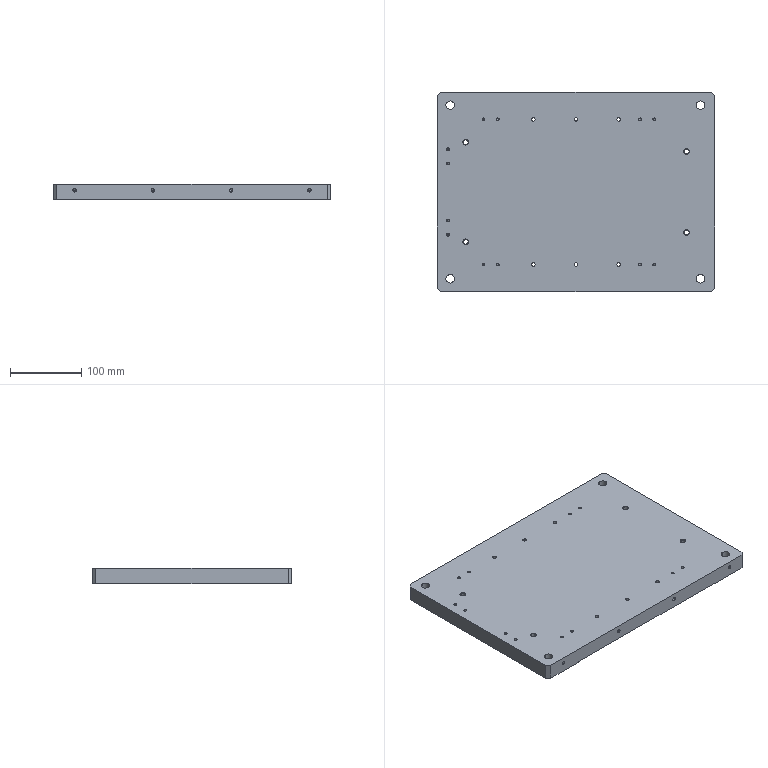NC program | NX | posted with a generic post | part box 390 x 280 x 22 mm
Lines 1 to 1875 of 1943, first 1630 of 1861 lines:
N10 G17 G21 G94 G90
(FLOOR_WALL , TOOL : D20R0.8)
N12 T01 M6
N14 G54
N16 G17 G0 G90 X-210.5 Y142.499 S7500 M3
N18 G43 Z30. H1
N20 Z3.
N22 G94 G1 Z0. F1350.
N24 X-207.5
N26 X207.5
N28 Y132.583
N30 X-207.5
N32 Y122.668
N34 X207.5
N36 Y112.752
N38 X-207.5
N40 Y102.836
N42 X207.5
N44 Y92.921
N46 X-207.5
N48 Y83.005
N50 X207.5
N52 Y73.089
N54 X-207.5
N56 Y63.174
N58 X207.5
N60 Y53.258
N62 X-207.5
N64 Y43.342
N66 X207.5
N68 Y33.427
N70 X-207.5
N72 Y23.511
N74 X207.5
N76 Y13.595
N78 X-207.5
N80 Y3.68
N82 X207.5
N84 Y-6.236
N86 X-207.5
N88 Y-16.152
N90 X207.5
N92 Y-26.068
N94 X-207.5
N96 Y-35.983
N98 X207.5
N100 Y-45.899
N102 X-207.5
N104 Y-55.815
N106 X207.5
N108 Y-65.73
N110 X-207.5
N112 Y-75.646
N114 X207.5
N116 Y-85.562
N118 X-207.5
N120 Y-95.477
N122 X207.5
N124 Y-105.393
N126 X-207.5
N128 Y-115.309
N130 X207.5
N132 Y-125.224
N134 X-207.5
N136 Y-135.14
N138 X207.5
N140 X210.5
N142 Z3.
N144 G0 Z30.
N146 M5
(ZLEVEL_PROFILE_1 , TOOL : D6)
N148 T06 M6
N150 G54
N152 G17 G0 G90 X34.282 Y-143.1 S9500 M3
N154 G43 Z30. H6
N156 Z1.5
N158 G94 G1 X0. Z-0.297 F1000.
N160 X-190. F3000.
N162 G2 X-192.192 Y-142.192 R3.1
N164 G1 X-197.192 Y-137.192
N166 G2 X-198.1 Y-135. R3.1
N168 G1 Y135.
N170 G2 X-197.192 Y137.192 R3.1
N172 G1 X-192.192 Y142.192
N174 G2 X-190. Y143.1 R3.1
N176 G1 X190.
N178 G2 X192.192 Y142.192 R3.1
N180 G1 X197.192 Y137.192
N182 G2 X198.1 Y135. R3.1
N184 G1 Y-135.
N186 G2 X197.192 Y-137.192 R3.1
N188 G1 X192.192 Y-142.192
N190 G2 X190. Y-143.1 R3.1
N192 G1 X0.
N194 X-16.993 Z-0.593
N196 X-190.
N198 G2 X-192.192 Y-142.192 R3.1
N200 G1 X-197.192 Y-137.192
N202 G2 X-198.1 Y-135. R3.1
N204 G1 Y135.
N206 G2 X-197.192 Y137.192 R3.1
N208 G1 X-192.192 Y142.192
N210 G2 X-190. Y143.1 R3.1
N212 G1 X190.
N214 G2 X192.192 Y142.192 R3.1
N216 G1 X197.192 Y137.192
N218 G2 X198.1 Y135. R3.1
N220 G1 Y-135.
N222 G2 X197.192 Y-137.192 R3.1
N224 G1 X192.192 Y-142.192
N226 G2 X190. Y-143.1 R3.1
N228 G1 X0.
N230 X-16.993 Z-0.89
N232 X-190.
N234 G2 X-192.192 Y-142.192 R3.1
N236 G1 X-197.192 Y-137.192
N238 G2 X-198.1 Y-135. R3.1
N240 G1 Y135.
N242 G2 X-197.192 Y137.192 R3.1
N244 G1 X-192.192 Y142.192
N246 G2 X-190. Y143.1 R3.1
N248 G1 X190.
N250 G2 X192.192 Y142.192 R3.1
N252 G1 X197.192 Y137.192
N254 G2 X198.1 Y135. R3.1
N256 G1 Y-135.
N258 G2 X197.192 Y-137.192 R3.1
N260 G1 X192.192 Y-142.192
N262 G2 X190. Y-143.1 R3.1
N264 G1 X0.
N266 X-16.993 Z-1.186
N268 X-190.
N270 G2 X-192.192 Y-142.192 R3.1
N272 G1 X-197.192 Y-137.192
N274 G2 X-198.1 Y-135. R3.1
N276 G1 Y135.
N278 G2 X-197.192 Y137.192 R3.1
N280 G1 X-192.192 Y142.192
N282 G2 X-190. Y143.1 R3.1
N284 G1 X190.
N286 G2 X192.192 Y142.192 R3.1
N288 G1 X197.192 Y137.192
N290 G2 X198.1 Y135. R3.1
N292 G1 Y-135.
N294 G2 X197.192 Y-137.192 R3.1
N296 G1 X192.192 Y-142.192
N298 G2 X190. Y-143.1 R3.1
N300 G1 X0.
N302 X-16.993 Z-1.483
N304 X-190.
N306 G2 X-192.192 Y-142.192 R3.1
N308 G1 X-197.192 Y-137.192
N310 G2 X-198.1 Y-135. R3.1
N312 G1 Y135.
N314 G2 X-197.192 Y137.192 R3.1
N316 G1 X-192.192 Y142.192
N318 G2 X-190. Y143.1 R3.1
N320 G1 X190.
N322 G2 X192.192 Y142.192 R3.1
N324 G1 X197.192 Y137.192
N326 G2 X198.1 Y135. R3.1
N328 G1 Y-135.
N330 G2 X197.192 Y-137.192 R3.1
N332 G1 X192.192 Y-142.192
N334 G2 X190. Y-143.1 R3.1
N336 G1 X0.
N338 X-16.993 Z-1.78
N340 X-190.
N342 G2 X-192.192 Y-142.192 R3.1
N344 G1 X-197.192 Y-137.192
N346 G2 X-198.1 Y-135. R3.1
N348 G1 Y135.
N350 G2 X-197.192 Y137.192 R3.1
N352 G1 X-192.192 Y142.192
N354 G2 X-190. Y143.1 R3.1
N356 G1 X190.
N358 G2 X192.192 Y142.192 R3.1
N360 G1 X197.192 Y137.192
N362 G2 X198.1 Y135. R3.1
N364 G1 Y-135.
N366 G2 X197.192 Y-137.192 R3.1
N368 G1 X192.192 Y-142.192
N370 G2 X190. Y-143.1 R3.1
N372 G1 X0.
N374 X-16.993 Z-2.076
N376 X-190.
N378 G2 X-192.192 Y-142.192 R3.1
N380 G1 X-197.192 Y-137.192
N382 G2 X-198.1 Y-135. R3.1
N384 G1 Y135.
N386 G2 X-197.192 Y137.192 R3.1
N388 G1 X-192.192 Y142.192
N390 G2 X-190. Y143.1 R3.1
N392 G1 X190.
N394 G2 X192.192 Y142.192 R3.1
N396 G1 X197.192 Y137.192
N398 G2 X198.1 Y135. R3.1
N400 G1 Y-135.
N402 G2 X197.192 Y-137.192 R3.1
N404 G1 X192.192 Y-142.192
N406 G2 X190. Y-143.1 R3.1
N408 G1 X0.
N410 X-16.993 Z-2.373
N412 X-190.
N414 G2 X-192.192 Y-142.192 R3.1
N416 G1 X-197.192 Y-137.192
N418 G2 X-198.1 Y-135. R3.1
N420 G1 Y135.
N422 G2 X-197.192 Y137.192 R3.1
N424 G1 X-192.192 Y142.192
N426 G2 X-190. Y143.1 R3.1
N428 G1 X190.
N430 G2 X192.192 Y142.192 R3.1
N432 G1 X197.192 Y137.192
N434 G2 X198.1 Y135. R3.1
N436 G1 Y-135.
N438 G2 X197.192 Y-137.192 R3.1
N440 G1 X192.192 Y-142.192
N442 G2 X190. Y-143.1 R3.1
N444 G1 X0.
N446 X-16.993 Z-2.67
N448 X-190.
N450 G2 X-192.192 Y-142.192 R3.1
N452 G1 X-197.192 Y-137.192
N454 G2 X-198.1 Y-135. R3.1
N456 G1 Y135.
N458 G2 X-197.192 Y137.192 R3.1
N460 G1 X-192.192 Y142.192
N462 G2 X-190. Y143.1 R3.1
N464 G1 X190.
N466 G2 X192.192 Y142.192 R3.1
N468 G1 X197.192 Y137.192
N470 G2 X198.1 Y135. R3.1
N472 G1 Y-135.
N474 G2 X197.192 Y-137.192 R3.1
N476 G1 X192.192 Y-142.192
N478 G2 X190. Y-143.1 R3.1
N480 G1 X0.
N482 X-16.993 Z-2.966
N484 X-190.
N486 G2 X-192.192 Y-142.192 R3.1
N488 G1 X-197.192 Y-137.192
N490 G2 X-198.1 Y-135. R3.1
N492 G1 Y135.
N494 G2 X-197.192 Y137.192 R3.1
N496 G1 X-192.192 Y142.192
N498 G2 X-190. Y143.1 R3.1
N500 G1 X190.
N502 G2 X192.192 Y142.192 R3.1
N504 G1 X197.192 Y137.192
N506 G2 X198.1 Y135. R3.1
N508 G1 Y-135.
N510 G2 X197.192 Y-137.192 R3.1
N512 G1 X192.192 Y-142.192
N514 G2 X190. Y-143.1 R3.1
N516 G1 X0.
N518 X-16.993 Z-3.263
N520 X-190.
N522 G2 X-192.192 Y-142.192 R3.1
N524 G1 X-197.192 Y-137.192
N526 G2 X-198.1 Y-135. R3.1
N528 G1 Y135.
N530 G2 X-197.192 Y137.192 R3.1
N532 G1 X-192.192 Y142.192
N534 G2 X-190. Y143.1 R3.1
N536 G1 X190.
N538 G2 X192.192 Y142.192 R3.1
N540 G1 X197.192 Y137.192
N542 G2 X198.1 Y135. R3.1
N544 G1 Y-135.
N546 G2 X197.192 Y-137.192 R3.1
N548 G1 X192.192 Y-142.192
N550 G2 X190. Y-143.1 R3.1
N552 G1 X0.
N554 X-16.993 Z-3.559
N556 X-190.
N558 G2 X-192.192 Y-142.192 R3.1
N560 G1 X-197.192 Y-137.192
N562 G2 X-198.1 Y-135. R3.1
N564 G1 Y135.
N566 G2 X-197.192 Y137.192 R3.1
N568 G1 X-192.192 Y142.192
N570 G2 X-190. Y143.1 R3.1
N572 G1 X190.
N574 G2 X192.192 Y142.192 R3.1
N576 G1 X197.192 Y137.192
N578 G2 X198.1 Y135. R3.1
N580 G1 Y-135.
N582 G2 X197.192 Y-137.192 R3.1
N584 G1 X192.192 Y-142.192
N586 G2 X190. Y-143.1 R3.1
N588 G1 X0.
N590 X-16.993 Z-3.856
N592 X-190.
N594 G2 X-192.192 Y-142.192 R3.1
N596 G1 X-197.192 Y-137.192
N598 G2 X-198.1 Y-135. R3.1
N600 G1 Y135.
N602 G2 X-197.192 Y137.192 R3.1
N604 G1 X-192.192 Y142.192
N606 G2 X-190. Y143.1 R3.1
N608 G1 X190.
N610 G2 X192.192 Y142.192 R3.1
N612 G1 X197.192 Y137.192
N614 G2 X198.1 Y135. R3.1
N616 G1 Y-135.
N618 G2 X197.192 Y-137.192 R3.1
N620 G1 X192.192 Y-142.192
N622 G2 X190. Y-143.1 R3.1
N624 G1 X0.
N626 X-16.993 Z-4.153
N628 X-190.
N630 G2 X-192.192 Y-142.192 R3.1
N632 G1 X-197.192 Y-137.192
N634 G2 X-198.1 Y-135. R3.1
N636 G1 Y135.
N638 G2 X-197.192 Y137.192 R3.1
N640 G1 X-192.192 Y142.192
N642 G2 X-190. Y143.1 R3.1
N644 G1 X190.
N646 G2 X192.192 Y142.192 R3.1
N648 G1 X197.192 Y137.192
N650 G2 X198.1 Y135. R3.1
N652 G1 Y-135.
N654 G2 X197.192 Y-137.192 R3.1
N656 G1 X192.192 Y-142.192
N658 G2 X190. Y-143.1 R3.1
N660 G1 X0.
N662 X-16.993 Z-4.449
N664 X-190.
N666 G2 X-192.192 Y-142.192 R3.1
N668 G1 X-197.192 Y-137.192
N670 G2 X-198.1 Y-135. R3.1
N672 G1 Y135.
N674 G2 X-197.192 Y137.192 R3.1
N676 G1 X-192.192 Y142.192
N678 G2 X-190. Y143.1 R3.1
N680 G1 X190.
N682 G2 X192.192 Y142.192 R3.1
N684 G1 X197.192 Y137.192
N686 G2 X198.1 Y135. R3.1
N688 G1 Y-135.
N690 G2 X197.192 Y-137.192 R3.1
N692 G1 X192.192 Y-142.192
N694 G2 X190. Y-143.1 R3.1
N696 G1 X0.
N698 X-16.993 Z-4.746
N700 X-190.
N702 G2 X-192.192 Y-142.192 R3.1
N704 G1 X-197.192 Y-137.192
N706 G2 X-198.1 Y-135. R3.1
N708 G1 Y135.
N710 G2 X-197.192 Y137.192 R3.1
N712 G1 X-192.192 Y142.192
N714 G2 X-190. Y143.1 R3.1
N716 G1 X190.
N718 G2 X192.192 Y142.192 R3.1
N720 G1 X197.192 Y137.192
N722 G2 X198.1 Y135. R3.1
N724 G1 Y-135.
N726 G2 X197.192 Y-137.192 R3.1
N728 G1 X192.192 Y-142.192
N730 G2 X190. Y-143.1 R3.1
N732 G1 X0.
N734 X-16.993 Z-5.043
N736 X-190.
N738 G2 X-192.192 Y-142.192 R3.1
N740 G1 X-197.192 Y-137.192
N742 G2 X-198.1 Y-135. R3.1
N744 G1 Y135.
N746 G2 X-197.192 Y137.192 R3.1
N748 G1 X-192.192 Y142.192
N750 G2 X-190. Y143.1 R3.1
N752 G1 X190.
N754 G2 X192.192 Y142.192 R3.1
N756 G1 X197.192 Y137.192
N758 G2 X198.1 Y135. R3.1
N760 G1 Y-135.
N762 G2 X197.192 Y-137.192 R3.1
N764 G1 X192.192 Y-142.192
N766 G2 X190. Y-143.1 R3.1
N768 G1 X0.
N770 X-16.993 Z-5.339
N772 X-190.
N774 G2 X-192.192 Y-142.192 R3.1
N776 G1 X-197.192 Y-137.192
N778 G2 X-198.1 Y-135. R3.1
N780 G1 Y135.
N782 G2 X-197.192 Y137.192 R3.1
N784 G1 X-192.192 Y142.192
N786 G2 X-190. Y143.1 R3.1
N788 G1 X190.
N790 G2 X192.192 Y142.192 R3.1
N792 G1 X197.192 Y137.192
N794 G2 X198.1 Y135. R3.1
N796 G1 Y-135.
N798 G2 X197.192 Y-137.192 R3.1
N800 G1 X192.192 Y-142.192
N802 G2 X190. Y-143.1 R3.1
N804 G1 X0.
N806 X-16.993 Z-5.636
N808 X-190.
N810 G2 X-192.192 Y-142.192 R3.1
N812 G1 X-197.192 Y-137.192
N814 G2 X-198.1 Y-135. R3.1
N816 G1 Y135.
N818 G2 X-197.192 Y137.192 R3.1
N820 G1 X-192.192 Y142.192
N822 G2 X-190. Y143.1 R3.1
N824 G1 X190.
N826 G2 X192.192 Y142.192 R3.1
N828 G1 X197.192 Y137.192
N830 G2 X198.1 Y135. R3.1
N832 G1 Y-135.
N834 G2 X197.192 Y-137.192 R3.1
N836 G1 X192.192 Y-142.192
N838 G2 X190. Y-143.1 R3.1
N840 G1 X0.
N842 X-16.993 Z-5.932
N844 X-190.
N846 G2 X-192.192 Y-142.192 R3.1
N848 G1 X-197.192 Y-137.192
N850 G2 X-198.1 Y-135. R3.1
N852 G1 Y135.
N854 G2 X-197.192 Y137.192 R3.1
N856 G1 X-192.192 Y142.192
N858 G2 X-190. Y143.1 R3.1
N860 G1 X190.
N862 G2 X192.192 Y142.192 R3.1
N864 G1 X197.192 Y137.192
N866 G2 X198.1 Y135. R3.1
N868 G1 Y-135.
N870 G2 X197.192 Y-137.192 R3.1
N872 G1 X192.192 Y-142.192
N874 G2 X190. Y-143.1 R3.1
N876 G1 X0.
N878 X-16.993 Z-6.229
N880 X-190.
N882 G2 X-192.192 Y-142.192 R3.1
N884 G1 X-197.192 Y-137.192
N886 G2 X-198.1 Y-135. R3.1
N888 G1 Y135.
N890 G2 X-197.192 Y137.192 R3.1
N892 G1 X-192.192 Y142.192
N894 G2 X-190. Y143.1 R3.1
N896 G1 X190.
N898 G2 X192.192 Y142.192 R3.1
N900 G1 X197.192 Y137.192
N902 G2 X198.1 Y135. R3.1
N904 G1 Y-135.
N906 G2 X197.192 Y-137.192 R3.1
N908 G1 X192.192 Y-142.192
N910 G2 X190. Y-143.1 R3.1
N912 G1 X0.
N914 X-16.993 Z-6.526
N916 X-190.
N918 G2 X-192.192 Y-142.192 R3.1
N920 G1 X-197.192 Y-137.192
N922 G2 X-198.1 Y-135. R3.1
N924 G1 Y135.
N926 G2 X-197.192 Y137.192 R3.1
N928 G1 X-192.192 Y142.192
N930 G2 X-190. Y143.1 R3.1
N932 G1 X190.
N934 G2 X192.192 Y142.192 R3.1
N936 G1 X197.192 Y137.192
N938 G2 X198.1 Y135. R3.1
N940 G1 Y-135.
N942 G2 X197.192 Y-137.192 R3.1
N944 G1 X192.192 Y-142.192
N946 G2 X190. Y-143.1 R3.1
N948 G1 X0.
N950 X-16.993 Z-6.822
N952 X-190.
N954 G2 X-192.192 Y-142.192 R3.1
N956 G1 X-197.192 Y-137.192
N958 G2 X-198.1 Y-135. R3.1
N960 G1 Y135.
N962 G2 X-197.192 Y137.192 R3.1
N964 G1 X-192.192 Y142.192
N966 G2 X-190. Y143.1 R3.1
N968 G1 X190.
N970 G2 X192.192 Y142.192 R3.1
N972 G1 X197.192 Y137.192
N974 G2 X198.1 Y135. R3.1
N976 G1 Y-135.
N978 G2 X197.192 Y-137.192 R3.1
N980 G1 X192.192 Y-142.192
N982 G2 X190. Y-143.1 R3.1
N984 G1 X0.
N986 X-16.993 Z-7.119
N988 X-190.
N990 G2 X-192.192 Y-142.192 R3.1
N992 G1 X-197.192 Y-137.192
N994 G2 X-198.1 Y-135. R3.1
N996 G1 Y135.
N998 G2 X-197.192 Y137.192 R3.1
N1000 G1 X-192.192 Y142.192
N1002 G2 X-190. Y143.1 R3.1
N1004 G1 X190.
N1006 G2 X192.192 Y142.192 R3.1
N1008 G1 X197.192 Y137.192
N1010 G2 X198.1 Y135. R3.1
N1012 G1 Y-135.
N1014 G2 X197.192 Y-137.192 R3.1
N1016 G1 X192.192 Y-142.192
N1018 G2 X190. Y-143.1 R3.1
N1020 G1 X0.
N1022 X-16.993 Z-7.416
N1024 X-190.
N1026 G2 X-192.192 Y-142.192 R3.1
N1028 G1 X-197.192 Y-137.192
N1030 G2 X-198.1 Y-135. R3.1
N1032 G1 Y135.
N1034 G2 X-197.192 Y137.192 R3.1
N1036 G1 X-192.192 Y142.192
N1038 G2 X-190. Y143.1 R3.1
N1040 G1 X190.
N1042 G2 X192.192 Y142.192 R3.1
N1044 G1 X197.192 Y137.192
N1046 G2 X198.1 Y135. R3.1
N1048 G1 Y-135.
N1050 G2 X197.192 Y-137.192 R3.1
N1052 G1 X192.192 Y-142.192
N1054 G2 X190. Y-143.1 R3.1
N1056 G1 X0.
N1058 X-16.993 Z-7.712
N1060 X-190.
N1062 G2 X-192.192 Y-142.192 R3.1
N1064 G1 X-197.192 Y-137.192
N1066 G2 X-198.1 Y-135. R3.1
N1068 G1 Y135.
N1070 G2 X-197.192 Y137.192 R3.1
N1072 G1 X-192.192 Y142.192
N1074 G2 X-190. Y143.1 R3.1
N1076 G1 X190.
N1078 G2 X192.192 Y142.192 R3.1
N1080 G1 X197.192 Y137.192
N1082 G2 X198.1 Y135. R3.1
N1084 G1 Y-135.
N1086 G2 X197.192 Y-137.192 R3.1
N1088 G1 X192.192 Y-142.192
N1090 G2 X190. Y-143.1 R3.1
N1092 G1 X0.
N1094 X-16.993 Z-8.009
N1096 X-190.
N1098 G2 X-192.192 Y-142.192 R3.1
N1100 G1 X-197.192 Y-137.192
N1102 G2 X-198.1 Y-135. R3.1
N1104 G1 Y135.
N1106 G2 X-197.192 Y137.192 R3.1
N1108 G1 X-192.192 Y142.192
N1110 G2 X-190. Y143.1 R3.1
N1112 G1 X190.
N1114 G2 X192.192 Y142.192 R3.1
N1116 G1 X197.192 Y137.192
N1118 G2 X198.1 Y135. R3.1
N1120 G1 Y-135.
N1122 G2 X197.192 Y-137.192 R3.1
N1124 G1 X192.192 Y-142.192
N1126 G2 X190. Y-143.1 R3.1
N1128 G1 X0.
N1130 X-16.993 Z-8.305
N1132 X-190.
N1134 G2 X-192.192 Y-142.192 R3.1
N1136 G1 X-197.192 Y-137.192
N1138 G2 X-198.1 Y-135. R3.1
N1140 G1 Y135.
N1142 G2 X-197.192 Y137.192 R3.1
N1144 G1 X-192.192 Y142.192
N1146 G2 X-190. Y143.1 R3.1
N1148 G1 X190.
N1150 G2 X192.192 Y142.192 R3.1
N1152 G1 X197.192 Y137.192
N1154 G2 X198.1 Y135. R3.1
N1156 G1 Y-135.
N1158 G2 X197.192 Y-137.192 R3.1
N1160 G1 X192.192 Y-142.192
N1162 G2 X190. Y-143.1 R3.1
N1164 G1 X0.
N1166 X-16.993 Z-8.602
N1168 X-190.
N1170 G2 X-192.192 Y-142.192 R3.1
N1172 G1 X-197.192 Y-137.192
N1174 G2 X-198.1 Y-135. R3.1
N1176 G1 Y135.
N1178 G2 X-197.192 Y137.192 R3.1
N1180 G1 X-192.192 Y142.192
N1182 G2 X-190. Y143.1 R3.1
N1184 G1 X190.
N1186 G2 X192.192 Y142.192 R3.1
N1188 G1 X197.192 Y137.192
N1190 G2 X198.1 Y135. R3.1
N1192 G1 Y-135.
N1194 G2 X197.192 Y-137.192 R3.1
N1196 G1 X192.192 Y-142.192
N1198 G2 X190. Y-143.1 R3.1
N1200 G1 X0.
N1202 X-16.993 Z-8.899
N1204 X-190.
N1206 G2 X-192.192 Y-142.192 R3.1
N1208 G1 X-197.192 Y-137.192
N1210 G2 X-198.1 Y-135. R3.1
N1212 G1 Y135.
N1214 G2 X-197.192 Y137.192 R3.1
N1216 G1 X-192.192 Y142.192
N1218 G2 X-190. Y143.1 R3.1
N1220 G1 X190.
N1222 G2 X192.192 Y142.192 R3.1
N1224 G1 X197.192 Y137.192
N1226 G2 X198.1 Y135. R3.1
N1228 G1 Y-135.
N1230 G2 X197.192 Y-137.192 R3.1
N1232 G1 X192.192 Y-142.192
N1234 G2 X190. Y-143.1 R3.1
N1236 G1 X0.
N1238 X-16.993 Z-9.195
N1240 X-190.
N1242 G2 X-192.192 Y-142.192 R3.1
N1244 G1 X-197.192 Y-137.192
N1246 G2 X-198.1 Y-135. R3.1
N1248 G1 Y135.
N1250 G2 X-197.192 Y137.192 R3.1
N1252 G1 X-192.192 Y142.192
N1254 G2 X-190. Y143.1 R3.1
N1256 G1 X190.
N1258 G2 X192.192 Y142.192 R3.1
N1260 G1 X197.192 Y137.192
N1262 G2 X198.1 Y135. R3.1
N1264 G1 Y-135.
N1266 G2 X197.192 Y-137.192 R3.1
N1268 G1 X192.192 Y-142.192
N1270 G2 X190. Y-143.1 R3.1
N1272 G1 X0.
N1274 X-16.993 Z-9.492
N1276 X-190.
N1278 G2 X-192.192 Y-142.192 R3.1
N1280 G1 X-197.192 Y-137.192
N1282 G2 X-198.1 Y-135. R3.1
N1284 G1 Y135.
N1286 G2 X-197.192 Y137.192 R3.1
N1288 G1 X-192.192 Y142.192
N1290 G2 X-190. Y143.1 R3.1
N1292 G1 X190.
N1294 G2 X192.192 Y142.192 R3.1
N1296 G1 X197.192 Y137.192
N1298 G2 X198.1 Y135. R3.1
N1300 G1 Y-135.
N1302 G2 X197.192 Y-137.192 R3.1
N1304 G1 X192.192 Y-142.192
N1306 G2 X190. Y-143.1 R3.1
N1308 G1 X0.
N1310 X-16.993 Z-9.789
N1312 X-190.
N1314 G2 X-192.192 Y-142.192 R3.1
N1316 G1 X-197.192 Y-137.192
N1318 G2 X-198.1 Y-135. R3.1
N1320 G1 Y135.
N1322 G2 X-197.192 Y137.192 R3.1
N1324 G1 X-192.192 Y142.192
N1326 G2 X-190. Y143.1 R3.1
N1328 G1 X190.
N1330 G2 X192.192 Y142.192 R3.1
N1332 G1 X197.192 Y137.192
N1334 G2 X198.1 Y135. R3.1
N1336 G1 Y-135.
N1338 G2 X197.192 Y-137.192 R3.1
N1340 G1 X192.192 Y-142.192
N1342 G2 X190. Y-143.1 R3.1
N1344 G1 X0.
N1346 X-16.993 Z-10.085
N1348 X-190.
N1350 G2 X-192.192 Y-142.192 R3.1
N1352 G1 X-197.192 Y-137.192
N1354 G2 X-198.1 Y-135. R3.1
N1356 G1 Y135.
N1358 G2 X-197.192 Y137.192 R3.1
N1360 G1 X-192.192 Y142.192
N1362 G2 X-190. Y143.1 R3.1
N1364 G1 X190.
N1366 G2 X192.192 Y142.192 R3.1
N1368 G1 X197.192 Y137.192
N1370 G2 X198.1 Y135. R3.1
N1372 G1 Y-135.
N1374 G2 X197.192 Y-137.192 R3.1
N1376 G1 X192.192 Y-142.192
N1378 G2 X190. Y-143.1 R3.1
N1380 G1 X0.
N1382 X-16.993 Z-10.382
N1384 X-190.
N1386 G2 X-192.192 Y-142.192 R3.1
N1388 G1 X-197.192 Y-137.192
N1390 G2 X-198.1 Y-135. R3.1
N1392 G1 Y135.
N1394 G2 X-197.192 Y137.192 R3.1
N1396 G1 X-192.192 Y142.192
N1398 G2 X-190. Y143.1 R3.1
N1400 G1 X190.
N1402 G2 X192.192 Y142.192 R3.1
N1404 G1 X197.192 Y137.192
N1406 G2 X198.1 Y135. R3.1
N1408 G1 Y-135.
N1410 G2 X197.192 Y-137.192 R3.1
N1412 G1 X192.192 Y-142.192
N1414 G2 X190. Y-143.1 R3.1
N1416 G1 X0.
N1418 X-16.993 Z-10.678
N1420 X-190.
N1422 G2 X-192.192 Y-142.192 R3.1
N1424 G1 X-197.192 Y-137.192
N1426 G2 X-198.1 Y-135. R3.1
N1428 G1 Y135.
N1430 G2 X-197.192 Y137.192 R3.1
N1432 G1 X-192.192 Y142.192
N1434 G2 X-190. Y143.1 R3.1
N1436 G1 X190.
N1438 G2 X192.192 Y142.192 R3.1
N1440 G1 X197.192 Y137.192
N1442 G2 X198.1 Y135. R3.1
N1444 G1 Y-135.
N1446 G2 X197.192 Y-137.192 R3.1
N1448 G1 X192.192 Y-142.192
N1450 G2 X190. Y-143.1 R3.1
N1452 G1 X0.
N1454 X-16.993 Z-10.975
N1456 X-190.
N1458 G2 X-192.192 Y-142.192 R3.1
N1460 G1 X-197.192 Y-137.192
N1462 G2 X-198.1 Y-135. R3.1
N1464 G1 Y135.
N1466 G2 X-197.192 Y137.192 R3.1
N1468 G1 X-192.192 Y142.192
N1470 G2 X-190. Y143.1 R3.1
N1472 G1 X190.
N1474 G2 X192.192 Y142.192 R3.1
N1476 G1 X197.192 Y137.192
N1478 G2 X198.1 Y135. R3.1
N1480 G1 Y-135.
N1482 G2 X197.192 Y-137.192 R3.1
N1484 G1 X192.192 Y-142.192
N1486 G2 X190. Y-143.1 R3.1
N1488 G1 X0.
N1490 X-16.993 Z-11.272
N1492 X-190.
N1494 G2 X-192.192 Y-142.192 R3.1
N1496 G1 X-197.192 Y-137.192
N1498 G2 X-198.1 Y-135. R3.1
N1500 G1 Y135.
N1502 G2 X-197.192 Y137.192 R3.1
N1504 G1 X-192.192 Y142.192
N1506 G2 X-190. Y143.1 R3.1
N1508 G1 X190.
N1510 G2 X192.192 Y142.192 R3.1
N1512 G1 X197.192 Y137.192
N1514 G2 X198.1 Y135. R3.1
N1516 G1 Y-135.
N1518 G2 X197.192 Y-137.192 R3.1
N1520 G1 X192.192 Y-142.192
N1522 G2 X190. Y-143.1 R3.1
N1524 G1 X0.
N1526 X-16.993 Z-11.568
N1528 X-190.
N1530 G2 X-192.192 Y-142.192 R3.1
N1532 G1 X-197.192 Y-137.192
N1534 G2 X-198.1 Y-135. R3.1
N1536 G1 Y135.
N1538 G2 X-197.192 Y137.192 R3.1
N1540 G1 X-192.192 Y142.192
N1542 G2 X-190. Y143.1 R3.1
N1544 G1 X190.
N1546 G2 X192.192 Y142.192 R3.1
N1548 G1 X197.192 Y137.192
N1550 G2 X198.1 Y135. R3.1
N1552 G1 Y-135.
N1554 G2 X197.192 Y-137.192 R3.1
N1556 G1 X192.192 Y-142.192
N1558 G2 X190. Y-143.1 R3.1
N1560 G1 X0.
N1562 X-16.993 Z-11.865
N1564 X-190.
N1566 G2 X-192.192 Y-142.192 R3.1
N1568 G1 X-197.192 Y-137.192
N1570 G2 X-198.1 Y-135. R3.1
N1572 G1 Y135.
N1574 G2 X-197.192 Y137.192 R3.1
N1576 G1 X-192.192 Y142.192
N1578 G2 X-190. Y143.1 R3.1
N1580 G1 X190.
N1582 G2 X192.192 Y142.192 R3.1
N1584 G1 X197.192 Y137.192
N1586 G2 X198.1 Y135. R3.1
N1588 G1 Y-135.
N1590 G2 X197.192 Y-137.192 R3.1
N1592 G1 X192.192 Y-142.192
N1594 G2 X190. Y-143.1 R3.1
N1596 G1 X0.
N1598 X-16.993 Z-12.161
N1600 X-190.
N1602 G2 X-192.192 Y-142.192 R3.1
N1604 G1 X-197.192 Y-137.192
N1606 G2 X-198.1 Y-135. R3.1
N1608 G1 Y135.
N1610 G2 X-197.192 Y137.192 R3.1
N1612 G1 X-192.192 Y142.192
N1614 G2 X-190. Y143.1 R3.1
N1616 G1 X190.
N1618 G2 X192.192 Y142.192 R3.1
N1620 G1 X197.192 Y137.192
N1622 G2 X198.1 Y135. R3.1
N1624 G1 Y-135.
N1626 G2 X197.192 Y-137.192 R3.1
N1628 G1 X192.192 Y-142.192
N1630 G2 X190. Y-143.1 R3.1
N1632 G1 X0.
N1634 X-16.993 Z-12.458
N1636 X-190.
N1638 G2 X-192.192 Y-142.192 R3.1
N1640 G1 X-197.192 Y-137.192
N1642 G2 X-198.1 Y-135. R3.1
N1644 G1 Y135.
N1646 G2 X-197.192 Y137.192 R3.1
N1648 G1 X-192.192 Y142.192
N1650 G2 X-190. Y143.1 R3.1
N1652 G1 X190.
N1654 G2 X192.192 Y142.192 R3.1
N1656 G1 X197.192 Y137.192
N1658 G2 X198.1 Y135. R3.1
N1660 G1 Y-135.
N1662 G2 X197.192 Y-137.192 R3.1
N1664 G1 X192.192 Y-142.192
N1666 G2 X190. Y-143.1 R3.1
N1668 G1 X0.
N1670 X-16.993 Z-12.755
N1672 X-190.
N1674 G2 X-192.192 Y-142.192 R3.1
N1676 G1 X-197.192 Y-137.192
N1678 G2 X-198.1 Y-135. R3.1
N1680 G1 Y135.
N1682 G2 X-197.192 Y137.192 R3.1
N1684 G1 X-192.192 Y142.192
N1686 G2 X-190. Y143.1 R3.1
N1688 G1 X190.
N1690 G2 X192.192 Y142.192 R3.1
N1692 G1 X197.192 Y137.192
N1694 G2 X198.1 Y135. R3.1
N1696 G1 Y-135.
N1698 G2 X197.192 Y-137.192 R3.1
N1700 G1 X192.192 Y-142.192
N1702 G2 X190. Y-143.1 R3.1
N1704 G1 X0.
N1706 X-16.993 Z-13.051
N1708 X-190.
N1710 G2 X-192.192 Y-142.192 R3.1
N1712 G1 X-197.192 Y-137.192
N1714 G2 X-198.1 Y-135. R3.1
N1716 G1 Y135.
N1718 G2 X-197.192 Y137.192 R3.1
N1720 G1 X-192.192 Y142.192
N1722 G2 X-190. Y143.1 R3.1
N1724 G1 X190.
N1726 G2 X192.192 Y142.192 R3.1
N1728 G1 X197.192 Y137.192
N1730 G2 X198.1 Y135. R3.1
N1732 G1 Y-135.
N1734 G2 X197.192 Y-137.192 R3.1
N1736 G1 X192.192 Y-142.192
N1738 G2 X190. Y-143.1 R3.1
N1740 G1 X0.
N1742 X-16.993 Z-13.348
N1744 X-190.
N1746 G2 X-192.192 Y-142.192 R3.1
N1748 G1 X-197.192 Y-137.192
N1750 G2 X-198.1 Y-135. R3.1
N1752 G1 Y135.
N1754 G2 X-197.192 Y137.192 R3.1
N1756 G1 X-192.192 Y142.192
N1758 G2 X-190. Y143.1 R3.1
N1760 G1 X190.
N1762 G2 X192.192 Y142.192 R3.1
N1764 G1 X197.192 Y137.192
N1766 G2 X198.1 Y135. R3.1
N1768 G1 Y-135.
N1770 G2 X197.192 Y-137.192 R3.1
N1772 G1 X192.192 Y-142.192
N1774 G2 X190. Y-143.1 R3.1
N1776 G1 X0.
N1778 X-16.993 Z-13.645
N1780 X-190.
N1782 G2 X-192.192 Y-142.192 R3.1
N1784 G1 X-197.192 Y-137.192
N1786 G2 X-198.1 Y-135. R3.1
N1788 G1 Y135.
N1790 G2 X-197.192 Y137.192 R3.1
N1792 G1 X-192.192 Y142.192
N1794 G2 X-190. Y143.1 R3.1
N1796 G1 X190.
N1798 G2 X192.192 Y142.192 R3.1
N1800 G1 X197.192 Y137.192
N1802 G2 X198.1 Y135. R3.1
N1804 G1 Y-135.
N1806 G2 X197.192 Y-137.192 R3.1
N1808 G1 X192.192 Y-142.192
N1810 G2 X190. Y-143.1 R3.1
N1812 G1 X0.
N1814 X-16.993 Z-13.941
N1816 X-190.
N1818 G2 X-192.192 Y-142.192 R3.1
N1820 G1 X-197.192 Y-137.192
N1822 G2 X-198.1 Y-135. R3.1
N1824 G1 Y135.
N1826 G2 X-197.192 Y137.192 R3.1
N1828 G1 X-192.192 Y142.192
N1830 G2 X-190. Y143.1 R3.1
N1832 G1 X190.
N1834 G2 X192.192 Y142.192 R3.1
N1836 G1 X197.192 Y137.192
N1838 G2 X198.1 Y135. R3.1
N1840 G1 Y-135.
N1842 G2 X197.192 Y-137.192 R3.1
N1844 G1 X192.192 Y-142.192
N1846 G2 X190. Y-143.1 R3.1
N1848 G1 X0.
N1850 X-16.993 Z-14.238
N1852 X-190.
N1854 G2 X-192.192 Y-142.192 R3.1
N1856 G1 X-197.192 Y-137.192
N1858 G2 X-198.1 Y-135. R3.1
N1860 G1 Y135.
N1862 G2 X-197.192 Y137.192 R3.1
N1864 G1 X-192.192 Y142.192
N1866 G2 X-190. Y143.1 R3.1
N1868 G1 X190.
N1870 G2 X192.192 Y142.192 R3.1
N1872 G1 X197.192 Y137.192
N1874 G2 X198.1 Y135. R3.1
N1876 G1 Y-135.
N1878 G2 X197.192 Y-137.192 R3.1
N1880 G1 X192.192 Y-142.192
N1882 G2 X190. Y-143.1 R3.1
N1884 G1 X0.
N1886 X-16.993 Z-14.534
N1888 X-190.
N1890 G2 X-192.192 Y-142.192 R3.1
N1892 G1 X-197.192 Y-137.192
N1894 G2 X-198.1 Y-135. R3.1
N1896 G1 Y135.
N1898 G2 X-197.192 Y137.192 R3.1
N1900 G1 X-192.192 Y142.192
N1902 G2 X-190. Y143.1 R3.1
N1904 G1 X190.
N1906 G2 X192.192 Y142.192 R3.1
N1908 G1 X197.192 Y137.192
N1910 G2 X198.1 Y135. R3.1
N1912 G1 Y-135.
N1914 G2 X197.192 Y-137.192 R3.1
N1916 G1 X192.192 Y-142.192
N1918 G2 X190. Y-143.1 R3.1
N1920 G1 X0.
N1922 X-16.993 Z-14.831
N1924 X-190.
N1926 G2 X-192.192 Y-142.192 R3.1
N1928 G1 X-197.192 Y-137.192
N1930 G2 X-198.1 Y-135. R3.1
N1932 G1 Y135.
N1934 G2 X-197.192 Y137.192 R3.1
N1936 G1 X-192.192 Y142.192
N1938 G2 X-190. Y143.1 R3.1
N1940 G1 X190.
N1942 G2 X192.192 Y142.192 R3.1
N1944 G1 X197.192 Y137.192
N1946 G2 X198.1 Y135. R3.1
N1948 G1 Y-135.
N1950 G2 X197.192 Y-137.192 R3.1
N1952 G1 X192.192 Y-142.192
N1954 G2 X190. Y-143.1 R3.1
N1956 G1 X0.
N1958 X-16.993 Z-15.128
N1960 X-190.
N1962 G2 X-192.192 Y-142.192 R3.1
N1964 G1 X-197.192 Y-137.192
N1966 G2 X-198.1 Y-135. R3.1
N1968 G1 Y135.
N1970 G2 X-197.192 Y137.192 R3.1
N1972 G1 X-192.192 Y142.192
N1974 G2 X-190. Y143.1 R3.1
N1976 G1 X190.
N1978 G2 X192.192 Y142.192 R3.1
N1980 G1 X197.192 Y137.192
N1982 G2 X198.1 Y135. R3.1
N1984 G1 Y-135.
N1986 G2 X197.192 Y-137.192 R3.1
N1988 G1 X192.192 Y-142.192
N1990 G2 X190. Y-143.1 R3.1
N1992 G1 X0.
N1994 X-16.993 Z-15.424
N1996 X-190.
N1998 G2 X-192.192 Y-142.192 R3.1
N2000 G1 X-197.192 Y-137.192
N2002 G2 X-198.1 Y-135. R3.1
N2004 G1 Y135.
N2006 G2 X-197.192 Y137.192 R3.1
N2008 G1 X-192.192 Y142.192
N2010 G2 X-190. Y143.1 R3.1
N2012 G1 X190.
N2014 G2 X192.192 Y142.192 R3.1
N2016 G1 X197.192 Y137.192
N2018 G2 X198.1 Y135. R3.1
N2020 G1 Y-135.
N2022 G2 X197.192 Y-137.192 R3.1
N2024 G1 X192.192 Y-142.192
N2026 G2 X190. Y-143.1 R3.1
N2028 G1 X0.
N2030 X-16.993 Z-15.721
N2032 X-190.
N2034 G2 X-192.192 Y-142.192 R3.1
N2036 G1 X-197.192 Y-137.192
N2038 G2 X-198.1 Y-135. R3.1
N2040 G1 Y135.
N2042 G2 X-197.192 Y137.192 R3.1
N2044 G1 X-192.192 Y142.192
N2046 G2 X-190. Y143.1 R3.1
N2048 G1 X190.
N2050 G2 X192.192 Y142.192 R3.1
N2052 G1 X197.192 Y137.192
N2054 G2 X198.1 Y135. R3.1
N2056 G1 Y-135.
N2058 G2 X197.192 Y-137.192 R3.1
N2060 G1 X192.192 Y-142.192
N2062 G2 X190. Y-143.1 R3.1
N2064 G1 X0.
N2066 X-16.993 Z-16.018
N2068 X-190.
N2070 G2 X-192.192 Y-142.192 R3.1
N2072 G1 X-197.192 Y-137.192
N2074 G2 X-198.1 Y-135. R3.1
N2076 G1 Y135.
N2078 G2 X-197.192 Y137.192 R3.1
N2080 G1 X-192.192 Y142.192
N2082 G2 X-190. Y143.1 R3.1
N2084 G1 X190.
N2086 G2 X192.192 Y142.192 R3.1
N2088 G1 X197.192 Y137.192
N2090 G2 X198.1 Y135. R3.1
N2092 G1 Y-135.
N2094 G2 X197.192 Y-137.192 R3.1
N2096 G1 X192.192 Y-142.192
N2098 G2 X190. Y-143.1 R3.1
N2100 G1 X0.
N2102 X-16.993 Z-16.314
N2104 X-190.
N2106 G2 X-192.192 Y-142.192 R3.1
N2108 G1 X-197.192 Y-137.192
N2110 G2 X-198.1 Y-135. R3.1
N2112 G1 Y135.
N2114 G2 X-197.192 Y137.192 R3.1
N2116 G1 X-192.192 Y142.192
N2118 G2 X-190. Y143.1 R3.1
N2120 G1 X190.
N2122 G2 X192.192 Y142.192 R3.1
N2124 G1 X197.192 Y137.192
N2126 G2 X198.1 Y135. R3.1
N2128 G1 Y-135.
N2130 G2 X197.192 Y-137.192 R3.1
N2132 G1 X192.192 Y-142.192
N2134 G2 X190. Y-143.1 R3.1
N2136 G1 X0.
N2138 X-16.993 Z-16.611
N2140 X-190.
N2142 G2 X-192.192 Y-142.192 R3.1
N2144 G1 X-197.192 Y-137.192
N2146 G2 X-198.1 Y-135. R3.1
N2148 G1 Y135.
N2150 G2 X-197.192 Y137.192 R3.1
N2152 G1 X-192.192 Y142.192
N2154 G2 X-190. Y143.1 R3.1
N2156 G1 X190.
N2158 G2 X192.192 Y142.192 R3.1
N2160 G1 X197.192 Y137.192
N2162 G2 X198.1 Y135. R3.1
N2164 G1 Y-135.
N2166 G2 X197.192 Y-137.192 R3.1
N2168 G1 X192.192 Y-142.192
N2170 G2 X190. Y-143.1 R3.1
N2172 G1 X0.
N2174 X-16.993 Z-16.907
N2176 X-190.
N2178 G2 X-192.192 Y-142.192 R3.1
N2180 G1 X-197.192 Y-137.192
N2182 G2 X-198.1 Y-135. R3.1
N2184 G1 Y135.
N2186 G2 X-197.192 Y137.192 R3.1
N2188 G1 X-192.192 Y142.192
N2190 G2 X-190. Y143.1 R3.1
N2192 G1 X190.
N2194 G2 X192.192 Y142.192 R3.1
N2196 G1 X197.192 Y137.192
N2198 G2 X198.1 Y135. R3.1
N2200 G1 Y-135.
N2202 G2 X197.192 Y-137.192 R3.1
N2204 G1 X192.192 Y-142.192
N2206 G2 X190. Y-143.1 R3.1
N2208 G1 X0.
N2210 X-16.993 Z-17.204
N2212 X-190.
N2214 G2 X-192.192 Y-142.192 R3.1
N2216 G1 X-197.192 Y-137.192
N2218 G2 X-198.1 Y-135. R3.1
N2220 G1 Y135.
N2222 G2 X-197.192 Y137.192 R3.1
N2224 G1 X-192.192 Y142.192
N2226 G2 X-190. Y143.1 R3.1
N2228 G1 X190.
N2230 G2 X192.192 Y142.192 R3.1
N2232 G1 X197.192 Y137.192
N2234 G2 X198.1 Y135. R3.1
N2236 G1 Y-135.
N2238 G2 X197.192 Y-137.192 R3.1
N2240 G1 X192.192 Y-142.192
N2242 G2 X190. Y-143.1 R3.1
N2244 G1 X0.
N2246 X-16.993 Z-17.501
N2248 X-190.
N2250 G2 X-192.192 Y-142.192 R3.1
N2252 G1 X-197.192 Y-137.192
N2254 G2 X-198.1 Y-135. R3.1
N2256 G1 Y135.
N2258 G2 X-197.192 Y137.192 R3.1
N2260 G1 X-192.192 Y142.192
N2262 G2 X-190. Y143.1 R3.1
N2264 G1 X190.
N2266 G2 X192.192 Y142.192 R3.1
N2268 G1 X197.192 Y137.192
N2270 G2 X198.1 Y135. R3.1
N2272 G1 Y-135.
N2274 G2 X197.192 Y-137.192 R3.1
N2276 G1 X192.192 Y-142.192
N2278 G2 X190. Y-143.1 R3.1
N2280 G1 X0.
N2282 X-16.993 Z-17.797
N2284 X-190.
N2286 G2 X-192.192 Y-142.192 R3.1
N2288 G1 X-197.192 Y-137.192
N2290 G2 X-198.1 Y-135. R3.1
N2292 G1 Y135.
N2294 G2 X-197.192 Y137.192 R3.1
N2296 G1 X-192.192 Y142.192
N2298 G2 X-190. Y143.1 R3.1
N2300 G1 X190.
N2302 G2 X192.192 Y142.192 R3.1
N2304 G1 X197.192 Y137.192
N2306 G2 X198.1 Y135. R3.1
N2308 G1 Y-135.
N2310 G2 X197.192 Y-137.192 R3.1
N2312 G1 X192.192 Y-142.192
N2314 G2 X190. Y-143.1 R3.1
N2316 G1 X0.
N2318 X-16.993 Z-18.094
N2320 X-190.
N2322 G2 X-192.192 Y-142.192 R3.1
N2324 G1 X-197.192 Y-137.192
N2326 G2 X-198.1 Y-135. R3.1
N2328 G1 Y135.
N2330 G2 X-197.192 Y137.192 R3.1
N2332 G1 X-192.192 Y142.192
N2334 G2 X-190. Y143.1 R3.1
N2336 G1 X190.
N2338 G2 X192.192 Y142.192 R3.1
N2340 G1 X197.192 Y137.192
N2342 G2 X198.1 Y135. R3.1
N2344 G1 Y-135.
N2346 G2 X197.192 Y-137.192 R3.1
N2348 G1 X192.192 Y-142.192
N2350 G2 X190. Y-143.1 R3.1
N2352 G1 X0.
N2354 X-16.993 Z-18.391
N2356 X-190.
N2358 G2 X-192.192 Y-142.192 R3.1
N2360 G1 X-197.192 Y-137.192
N2362 G2 X-198.1 Y-135. R3.1
N2364 G1 Y135.
N2366 G2 X-197.192 Y137.192 R3.1
N2368 G1 X-192.192 Y142.192
N2370 G2 X-190. Y143.1 R3.1
N2372 G1 X190.
N2374 G2 X192.192 Y142.192 R3.1
N2376 G1 X197.192 Y137.192
N2378 G2 X198.1 Y135. R3.1
N2380 G1 Y-135.
N2382 G2 X197.192 Y-137.192 R3.1
N2384 G1 X192.192 Y-142.192
N2386 G2 X190. Y-143.1 R3.1
N2388 G1 X0.
N2390 X-16.993 Z-18.687
N2392 X-190.
N2394 G2 X-192.192 Y-142.192 R3.1
N2396 G1 X-197.192 Y-137.192
N2398 G2 X-198.1 Y-135. R3.1
N2400 G1 Y135.
N2402 G2 X-197.192 Y137.192 R3.1
N2404 G1 X-192.192 Y142.192
N2406 G2 X-190. Y143.1 R3.1
N2408 G1 X190.
N2410 G2 X192.192 Y142.192 R3.1
N2412 G1 X197.192 Y137.192
N2414 G2 X198.1 Y135. R3.1
N2416 G1 Y-135.
N2418 G2 X197.192 Y-137.192 R3.1
N2420 G1 X192.192 Y-142.192
N2422 G2 X190. Y-143.1 R3.1
N2424 G1 X0.
N2426 X-16.993 Z-18.984
N2428 X-190.
N2430 G2 X-192.192 Y-142.192 R3.1
N2432 G1 X-197.192 Y-137.192
N2434 G2 X-198.1 Y-135. R3.1
N2436 G1 Y135.
N2438 G2 X-197.192 Y137.192 R3.1
N2440 G1 X-192.192 Y142.192
N2442 G2 X-190. Y143.1 R3.1
N2444 G1 X190.
N2446 G2 X192.192 Y142.192 R3.1
N2448 G1 X197.192 Y137.192
N2450 G2 X198.1 Y135. R3.1
N2452 G1 Y-135.
N2454 G2 X197.192 Y-137.192 R3.1
N2456 G1 X192.192 Y-142.192
N2458 G2 X190. Y-143.1 R3.1
N2460 G1 X0.
N2462 X-16.993 Z-19.28
N2464 X-190.
N2466 G2 X-192.192 Y-142.192 R3.1
N2468 G1 X-197.192 Y-137.192
N2470 G2 X-198.1 Y-135. R3.1
N2472 G1 Y135.
N2474 G2 X-197.192 Y137.192 R3.1
N2476 G1 X-192.192 Y142.192
N2478 G2 X-190. Y143.1 R3.1
N2480 G1 X190.
N2482 G2 X192.192 Y142.192 R3.1
N2484 G1 X197.192 Y137.192
N2486 G2 X198.1 Y135. R3.1
N2488 G1 Y-135.
N2490 G2 X197.192 Y-137.192 R3.1
N2492 G1 X192.192 Y-142.192
N2494 G2 X190. Y-143.1 R3.1
N2496 G1 X0.
N2498 X-16.993 Z-19.577
N2500 X-190.
N2502 G2 X-192.192 Y-142.192 R3.1
N2504 G1 X-197.192 Y-137.192
N2506 G2 X-198.1 Y-135. R3.1
N2508 G1 Y135.
N2510 G2 X-197.192 Y137.192 R3.1
N2512 G1 X-192.192 Y142.192
N2514 G2 X-190. Y143.1 R3.1
N2516 G1 X190.
N2518 G2 X192.192 Y142.192 R3.1
N2520 G1 X197.192 Y137.192
N2522 G2 X198.1 Y135. R3.1
N2524 G1 Y-135.
N2526 G2 X197.192 Y-137.192 R3.1
N2528 G1 X192.192 Y-142.192
N2530 G2 X190. Y-143.1 R3.1
N2532 G1 X0.
N2534 X-16.993 Z-19.874
N2536 X-190.
N2538 G2 X-192.192 Y-142.192 R3.1
N2540 G1 X-197.192 Y-137.192
N2542 G2 X-198.1 Y-135. R3.1
N2544 G1 Y135.
N2546 G2 X-197.192 Y137.192 R3.1
N2548 G1 X-192.192 Y142.192
N2550 G2 X-190. Y143.1 R3.1
N2552 G1 X190.
N2554 G2 X192.192 Y142.192 R3.1
N2556 G1 X197.192 Y137.192
N2558 G2 X198.1 Y135. R3.1
N2560 G1 Y-135.
N2562 G2 X197.192 Y-137.192 R3.1
N2564 G1 X192.192 Y-142.192
N2566 G2 X190. Y-143.1 R3.1
N2568 G1 X0.
N2570 X-16.993 Z-20.17
N2572 X-190.
N2574 G2 X-192.192 Y-142.192 R3.1
N2576 G1 X-197.192 Y-137.192
N2578 G2 X-198.1 Y-135. R3.1
N2580 G1 Y135.
N2582 G2 X-197.192 Y137.192 R3.1
N2584 G1 X-192.192 Y142.192
N2586 G2 X-190. Y143.1 R3.1
N2588 G1 X190.
N2590 G2 X192.192 Y142.192 R3.1
N2592 G1 X197.192 Y137.192
N2594 G2 X198.1 Y135. R3.1
N2596 G1 Y-135.
N2598 G2 X197.192 Y-137.192 R3.1
N2600 G1 X192.192 Y-142.192
N2602 G2 X190. Y-143.1 R3.1
N2604 G1 X0.
N2606 X-16.993 Z-20.467
N2608 X-190.
N2610 G2 X-192.192 Y-142.192 R3.1
N2612 G1 X-197.192 Y-137.192
N2614 G2 X-198.1 Y-135. R3.1
N2616 G1 Y135.
N2618 G2 X-197.192 Y137.192 R3.1
N2620 G1 X-192.192 Y142.192
N2622 G2 X-190. Y143.1 R3.1
N2624 G1 X190.
N2626 G2 X192.192 Y142.192 R3.1
N2628 G1 X197.192 Y137.192
N2630 G2 X198.1 Y135. R3.1
N2632 G1 Y-135.
N2634 G2 X197.192 Y-137.192 R3.1
N2636 G1 X192.192 Y-142.192
N2638 G2 X190. Y-143.1 R3.1
N2640 G1 X0.
N2642 X-16.993 Z-20.764
N2644 X-190.
N2646 G2 X-192.192 Y-142.192 R3.1
N2648 G1 X-197.192 Y-137.192
N2650 G2 X-198.1 Y-135. R3.1
N2652 G1 Y135.
N2654 G2 X-197.192 Y137.192 R3.1
N2656 G1 X-192.192 Y142.192
N2658 G2 X-190. Y143.1 R3.1
N2660 G1 X190.
N2662 G2 X192.192 Y142.192 R3.1
N2664 G1 X197.192 Y137.192
N2666 G2 X198.1 Y135. R3.1
N2668 G1 Y-135.
N2670 G2 X197.192 Y-137.192 R3.1
N2672 G1 X192.192 Y-142.192
N2674 G2 X190. Y-143.1 R3.1
N2676 G1 X0.
N2678 X-16.993 Z-21.06
N2680 X-190.
N2682 G2 X-192.192 Y-142.192 R3.1
N2684 G1 X-197.192 Y-137.192
N2686 G2 X-198.1 Y-135. R3.1
N2688 G1 Y135.
N2690 G2 X-197.192 Y137.192 R3.1
N2692 G1 X-192.192 Y142.192
N2694 G2 X-190. Y143.1 R3.1
N2696 G1 X190.
N2698 G2 X192.192 Y142.192 R3.1
N2700 G1 X197.192 Y137.192
N2702 G2 X198.1 Y135. R3.1
N2704 G1 Y-135.
N2706 G2 X197.192 Y-137.192 R3.1
N2708 G1 X192.192 Y-142.192
N2710 G2 X190. Y-143.1 R3.1
N2712 G1 X0.
N2714 X-16.993 Z-21.357
N2716 X-190.
N2718 G2 X-192.192 Y-142.192 R3.1
N2720 G1 X-197.192 Y-137.192
N2722 G2 X-198.1 Y-135. R3.1
N2724 G1 Y135.
N2726 G2 X-197.192 Y137.192 R3.1
N2728 G1 X-192.192 Y142.192
N2730 G2 X-190. Y143.1 R3.1
N2732 G1 X190.
N2734 G2 X192.192 Y142.192 R3.1
N2736 G1 X197.192 Y137.192
N2738 G2 X198.1 Y135. R3.1
N2740 G1 Y-135.
N2742 G2 X197.192 Y-137.192 R3.1
N2744 G1 X192.192 Y-142.192
N2746 G2 X190. Y-143.1 R3.1
N2748 G1 X0.
N2750 X-16.993 Z-21.653
N2752 X-190.
N2754 G2 X-192.192 Y-142.192 R3.1
N2756 G1 X-197.192 Y-137.192
N2758 G2 X-198.1 Y-135. R3.1
N2760 G1 Y135.
N2762 G2 X-197.192 Y137.192 R3.1
N2764 G1 X-192.192 Y142.192
N2766 G2 X-190. Y143.1 R3.1
N2768 G1 X190.
N2770 G2 X192.192 Y142.192 R3.1
N2772 G1 X197.192 Y137.192
N2774 G2 X198.1 Y135. R3.1
N2776 G1 Y-135.
N2778 G2 X197.192 Y-137.192 R3.1
N2780 G1 X192.192 Y-142.192
N2782 G2 X190. Y-143.1 R3.1
N2784 G1 X0.
N2786 X-16.993 Z-21.95
N2788 X-190.
N2790 G2 X-192.192 Y-142.192 R3.1
N2792 G1 X-197.192 Y-137.192
N2794 G2 X-198.1 Y-135. R3.1
N2796 G1 Y135.
N2798 G2 X-197.192 Y137.192 R3.1
N2800 G1 X-192.192 Y142.192
N2802 G2 X-190. Y143.1 R3.1
N2804 G1 X190.
N2806 G2 X192.192 Y142.192 R3.1
N2808 G1 X197.192 Y137.192
N2810 G2 X198.1 Y135. R3.1
N2812 G1 Y-135.
N2814 G2 X197.192 Y-137.192 R3.1
N2816 G1 X192.192 Y-142.192
N2818 G2 X190. Y-143.1 R3.1
N2820 G1 X-16.993
N2822 Z-20.45
N2824 G0 Z30.
(ZLEVEL_PROFILE_COPY , TOOL : D6)
N2826 X190.335 Y-143.102
N2828 Z-9.475
N2830 G1 Z-10.975 F1000.
N2832 G3 X190. Y-143. R0.6
N2834 G1 X-190. F1500.
N2836 G2 X-192.121 Y-142.121 R3.
N2838 G1 X-197.121 Y-137.121
N2840 G2 X-198. Y-135. R3.
N2842 G1 Y135.
N2844 G2 X-197.121 Y137.121 R3.
N2846 G1 X-192.121 Y142.121
N2848 G2 X-190. Y143. R3.
N2850 G1 X190.
N2852 G2 X192.121 Y142.121 R3.
N2854 G1 X197.121 Y137.121
N2856 G2 X198. Y135. R3.
N2858 G1 Y-135.
N2860 G2 X197.121 Y-137.121 R3.
N2862 G1 X192.121 Y-142.121
N2864 G2 X190. Y-143. R3.
N2866 G1 X-189.712 Z-17.603
N2868 X-190.012 Z-17.608
N2870 X-190.311 Y-142.984 Z-17.613
N2872 X-190.607 Y-142.938 Z-17.619
N2874 X-190.897 Y-142.863 Z-17.624
N2876 X-191.178 Y-142.759 Z-17.629
N2878 X-191.447 Y-142.628 Z-17.634
N2880 X-191.702 Y-142.47 Z-17.64
N2882 X-191.94 Y-142.289 Z-17.645
N2884 X-192.159 Y-142.084 Z-17.65
N2886 X-196.821 Y-137.422 Z-17.765
N2888 X-197.033 Y-137.21 Z-17.77
N2890 X-197.241 Y-136.994 Z-17.776
N2892 X-197.429 Y-136.761 Z-17.781
N2894 X-197.592 Y-136.51 Z-17.786
N2896 X-197.73 Y-136.244 Z-17.791
N2898 X-197.84 Y-135.965 Z-17.796
N2900 X-197.923 Y-135.677 Z-17.802
N2902 X-197.976 Y-135.382 Z-17.807
N2904 X-197.999 Y-135.084 Z-17.812
N2906 X-198. Y-134.784 Z-17.817
N2908 Y101.974 Z-21.95
N2910 Y135.
N2912 G2 X-197.121 Y137.121 R3.
N2914 G1 X-192.121 Y142.121
N2916 G2 X-190. Y143. R3.
N2918 G1 X190.
N2920 G2 X192.121 Y142.121 R3.
N2922 G1 X197.121 Y137.121
N2924 G2 X198. Y135. R3.
N2926 G1 Y-135.
N2928 G2 X197.121 Y-137.121 R3.
N2930 G1 X192.121 Y-142.121
N2932 G2 X190. Y-143. R3.
N2934 G1 X-190.
N2936 G2 X-192.121 Y-142.121 R3.
N2938 G1 X-197.121 Y-137.121
N2940 G2 X-198. Y-135. R3.
N2942 G1 Y101.974
N2944 G3 X-198.12 Y102.334 R0.6
N2946 G1 Z-20.45
N2948 G0 Z30.
(HOLE_MILLING , TOOL : D6)
N2950 X-177. Y122.
N2952 Z0.5
N2954 G3 X-175.5 Y120.5 R1.5 F1600.
N2956 X-174. Y122. R1.5
N2958 X-174. Y122. Z0.2 I-3. J0.
N2960 X-174. Y122. Z-0.1 I-3. J0.
N2962 X-174. Y122. Z-0.4 I-3. J0.
N2964 X-174. Y122. Z-0.7 I-3. J0.
N2966 X-174. Y122. Z-1. I-3. J0.
N2968 X-174. Y122. Z-1.3 I-3. J0.
N2970 X-174. Y122. Z-1.6 I-3. J0.
N2972 X-174. Y122. Z-1.9 I-3. J0.
N2974 X-174. Y122. Z-2.2 I-3. J0.
N2976 X-174. Y122. Z-2.5 I-3. J0.
N2978 X-174. Y122. Z-2.8 I-3. J0.
N2980 X-174. Y122. Z-3.1 I-3. J0.
N2982 X-174. Y122. Z-3.4 I-3. J0.
N2984 X-174. Y122. Z-3.7 I-3. J0.
N2986 X-174. Y122. Z-4. I-3. J0.
N2988 X-174. Y122. Z-4.3 I-3. J0.
N2990 X-174. Y122. Z-4.6 I-3. J0.
N2992 X-174. Y122. Z-4.9 I-3. J0.
N2994 X-174. Y122. Z-5.2 I-3. J0.
N2996 X-174. Y122. Z-5.5 I-3. J0.
N2998 X-174. Y122. Z-5.8 I-3. J0.
N3000 X-174. Y122. Z-6.1 I-3. J0.
N3002 X-174. Y122. Z-6.4 I-3. J0.
N3004 X-174. Y122. Z-6.7 I-3. J0.
N3006 X-174. Y122. Z-7. I-3. J0.
N3008 X-174. Y122. Z-7.3 I-3. J0.
N3010 X-174. Y122. Z-7.6 I-3. J0.
N3012 X-174. Y122. Z-7.9 I-3. J0.
N3014 X-174. Y122. Z-8.2 I-3. J0.
N3016 X-174. Y122. Z-8.5 I-3. J0.
N3018 X-174. Y122. Z-8.8 I-3. J0.
N3020 X-174. Y122. Z-9.1 I-3. J0.
N3022 X-174. Y122. Z-9.4 I-3. J0.
N3024 X-174. Y122. Z-9.7 I-3. J0.
N3026 X-174. Y122. Z-10. I-3. J0.
N3028 X-174. Y122. Z-10.3 I-3. J0.
N3030 X-174. Y122. Z-10.6 I-3. J0.
N3032 X-174. Y122. Z-10.9 I-3. J0.
N3034 X-174. Y122. Z-11.2 I-3. J0.
N3036 X-174. Y122. Z-11.5 I-3. J0.
N3038 X-174. Y122. Z-11.8 I-3. J0.
N3040 X-174. Y122. Z-12.1 I-3. J0.
N3042 X-174. Y122. Z-12.4 I-3. J0.
N3044 X-174. Y122. Z-12.7 I-3. J0.
N3046 X-174. Y122. Z-13. I-3. J0.
N3048 X-174. Y122. Z-13.3 I-3. J0.
N3050 X-174. Y122. Z-13.6 I-3. J0.
N3052 X-174. Y122. Z-13.9 I-3. J0.
N3054 X-174. Y122. Z-14.2 I-3. J0.
N3056 X-174. Y122. Z-14.5 I-3. J0.
N3058 X-174. Y122. Z-14.8 I-3. J0.
N3060 X-174. Y122. Z-15.1 I-3. J0.
N3062 X-174. Y122. Z-15.4 I-3. J0.
N3064 X-174. Y122. Z-15.7 I-3. J0.
N3066 X-174. Y122. Z-16. I-3. J0.
N3068 X-174. Y122. Z-16.3 I-3. J0.
N3070 X-174. Y122. Z-16.6 I-3. J0.
N3072 X-174. Y122. Z-16.9 I-3. J0.
N3074 X-174. Y122. Z-17.2 I-3. J0.
N3076 X-174. Y122. Z-17.5 I-3. J0.
N3078 X-174. Y122. Z-17.8 I-3. J0.
N3080 X-174. Y122. Z-18.1 I-3. J0.
N3082 X-174. Y122. Z-18.4 I-3. J0.
N3084 X-174. Y122. Z-18.7 I-3. J0.
N3086 X-174. Y122. Z-19. I-3. J0.
N3088 X-174. Y122. Z-19.3 I-3. J0.
N3090 X-174. Y122. Z-19.6 I-3. J0.
N3092 X-174. Y122. Z-19.9 I-3. J0.
N3094 X-174. Y122. Z-20.2 I-3. J0.
N3096 X-174. Y122. Z-20.5 I-3. J0.
N3098 X-174. Y122. Z-20.8 I-3. J0.
N3100 X-174. Y122. Z-21.1 I-3. J0.
N3102 X-174. Y122. Z-21.4 I-3. J0.
N3104 X-174. Y122. Z-21.7 I-3. J0.
N3106 X-175.5 Y119.402 Z-21.95 R-3.
N3108 X-174.402 Y123.5 R3.
N3110 X-175.5 Y119.402 R-3.
N3112 X-174.951 Y121.451 R1.5
N3114 X-177. Y122. R1.5
N3116 G0 Z30.
N3118 Y-122.
N3120 Z0.5
N3122 G3 X-175.5 Y-123.5 R1.5
N3124 X-174. Y-122. R1.5
N3126 X-174. Y-122. Z0.2 I-3. J0.
N3128 X-174. Y-122. Z-0.1 I-3. J0.
N3130 X-174. Y-122. Z-0.4 I-3. J0.
N3132 X-174. Y-122. Z-0.7 I-3. J0.
N3134 X-174. Y-122. Z-1. I-3. J0.
N3136 X-174. Y-122. Z-1.3 I-3. J0.
N3138 X-174. Y-122. Z-1.6 I-3. J0.
N3140 X-174. Y-122. Z-1.9 I-3. J0.
N3142 X-174. Y-122. Z-2.2 I-3. J0.
N3144 X-174. Y-122. Z-2.5 I-3. J0.
N3146 X-174. Y-122. Z-2.8 I-3. J0.
N3148 X-174. Y-122. Z-3.1 I-3. J0.
N3150 X-174. Y-122. Z-3.4 I-3. J0.
N3152 X-174. Y-122. Z-3.7 I-3. J0.
N3154 X-174. Y-122. Z-4. I-3. J0.
N3156 X-174. Y-122. Z-4.3 I-3. J0.
N3158 X-174. Y-122. Z-4.6 I-3. J0.
N3160 X-174. Y-122. Z-4.9 I-3. J0.
N3162 X-174. Y-122. Z-5.2 I-3. J0.
N3164 X-174. Y-122. Z-5.5 I-3. J0.
N3166 X-174. Y-122. Z-5.8 I-3. J0.
N3168 X-174. Y-122. Z-6.1 I-3. J0.
N3170 X-174. Y-122. Z-6.4 I-3. J0.
N3172 X-174. Y-122. Z-6.7 I-3. J0.
N3174 X-174. Y-122. Z-7. I-3. J0.
N3176 X-174. Y-122. Z-7.3 I-3. J0.
N3178 X-174. Y-122. Z-7.6 I-3. J0.
N3180 X-174. Y-122. Z-7.9 I-3. J0.
N3182 X-174. Y-122. Z-8.2 I-3. J0.
N3184 X-174. Y-122. Z-8.5 I-3. J0.
N3186 X-174. Y-122. Z-8.8 I-3. J0.
N3188 X-174. Y-122. Z-9.1 I-3. J0.
N3190 X-174. Y-122. Z-9.4 I-3. J0.
N3192 X-174. Y-122. Z-9.7 I-3. J0.
N3194 X-174. Y-122. Z-10. I-3. J0.
N3196 X-174. Y-122. Z-10.3 I-3. J0.
N3198 X-174. Y-122. Z-10.6 I-3. J0.
N3200 X-174. Y-122. Z-10.9 I-3. J0.
N3202 X-174. Y-122. Z-11.2 I-3. J0.
N3204 X-174. Y-122. Z-11.5 I-3. J0.
N3206 X-174. Y-122. Z-11.8 I-3. J0.
N3208 X-174. Y-122. Z-12.1 I-3. J0.
N3210 X-174. Y-122. Z-12.4 I-3. J0.
N3212 X-174. Y-122. Z-12.7 I-3. J0.
N3214 X-174. Y-122. Z-13. I-3. J0.
N3216 X-174. Y-122. Z-13.3 I-3. J0.
N3218 X-174. Y-122. Z-13.6 I-3. J0.
N3220 X-174. Y-122. Z-13.9 I-3. J0.
N3222 X-174. Y-122. Z-14.2 I-3. J0.
N3224 X-174. Y-122. Z-14.5 I-3. J0.
N3226 X-174. Y-122. Z-14.8 I-3. J0.
N3228 X-174. Y-122. Z-15.1 I-3. J0.
N3230 X-174. Y-122. Z-15.4 I-3. J0.
N3232 X-174. Y-122. Z-15.7 I-3. J0.
N3234 X-174. Y-122. Z-16. I-3. J0.
N3236 X-174. Y-122. Z-16.3 I-3. J0.
N3238 X-174. Y-122. Z-16.6 I-3. J0.
N3240 X-174. Y-122. Z-16.9 I-3. J0.
N3242 X-174. Y-122. Z-17.2 I-3. J0.
N3244 X-174. Y-122. Z-17.5 I-3. J0.
N3246 X-174. Y-122. Z-17.8 I-3. J0.
N3248 X-174. Y-122. Z-18.1 I-3. J0.
N3250 X-174. Y-122. Z-18.4 I-3. J0.
N3252 X-174. Y-122. Z-18.7 I-3. J0.
N3254 X-174. Y-122. Z-19. I-3. J0.
N3256 X-174. Y-122. Z-19.3 I-3. J0.
N3258 X-174. Y-122. Z-19.6 I-3. J0.
N3260 X-174. Y-122. Z-19.9 I-3. J0.